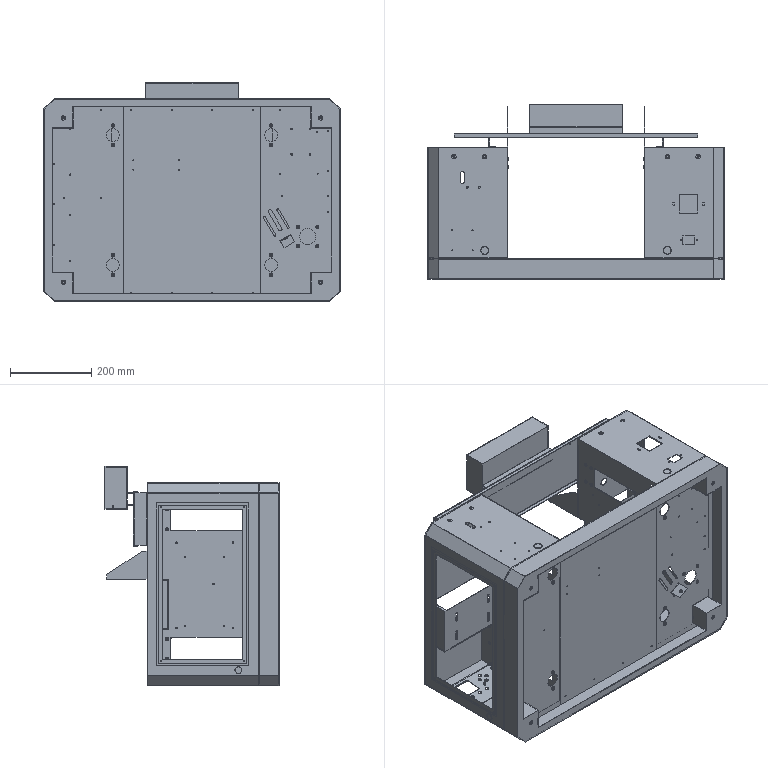Part | SolidWorks | 8 solids | 934 faces | box 730 x 429 x 540 mm | volume 2282239 mm3 | cylinder 508 | plane 390 | cone 36 | commonest cylinder face diameters 2.5 x138 3.3 x92 4.2 x58 7.9 x40 5 x34 8 x22